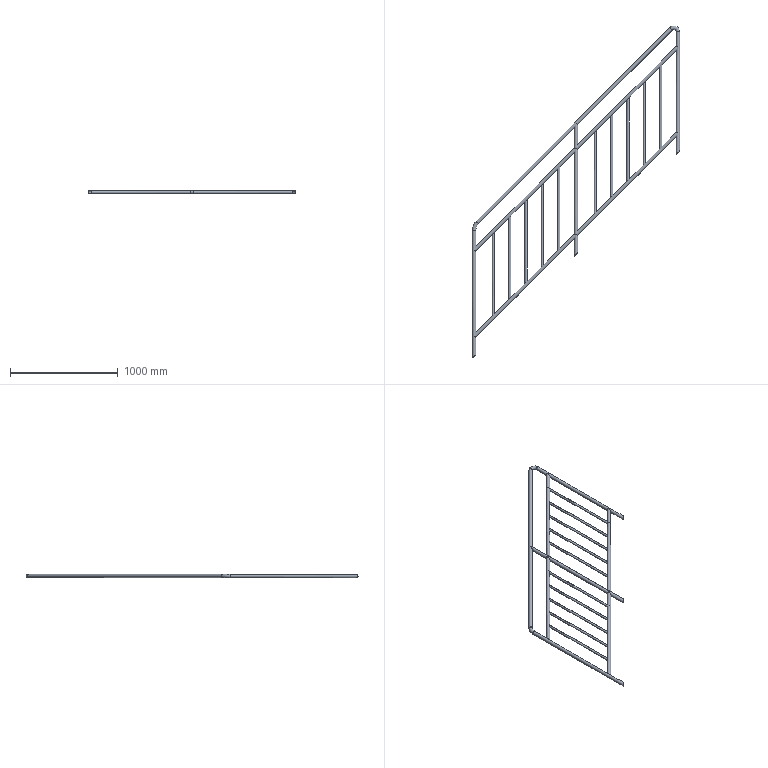Part | STEP file | PN_0014 stair guardrail A_Default<As Machined> | 20 solids | 80 faces | box 1927 x 3087 x 32 mm | volume 3023959 mm3 | cylinder 61 | plane 15 | torus 4 | commonest cylinder face diameters 32 x33 16 x10 20 x10 28 x8